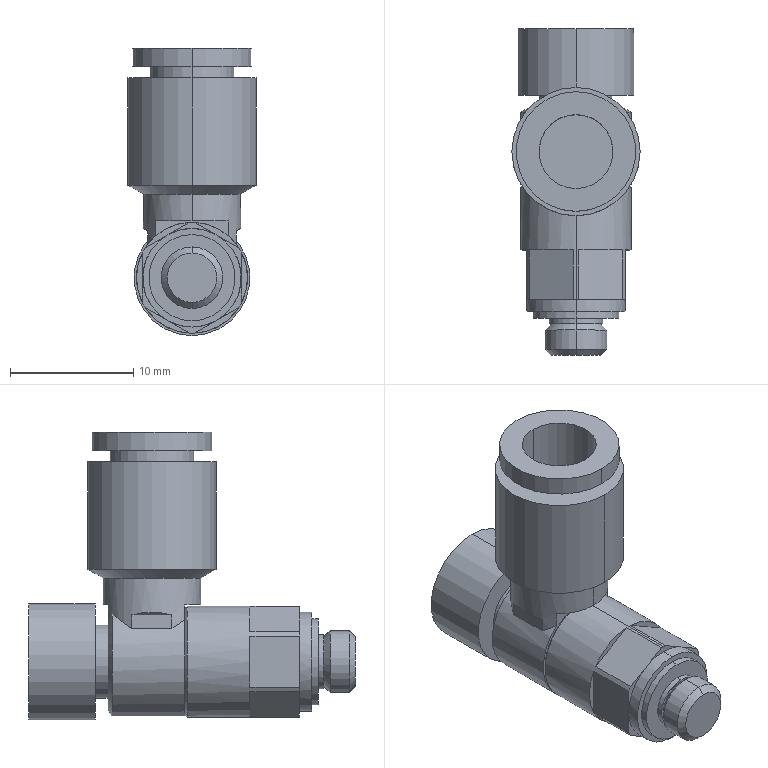Part | STEP file | speed control fitting AS1201FM-M5E-06A | 1 solid | 73 faces | box 10.4 x 26.5 x 23.3 mm | volume 2163 mm3 | plane 37 | cylinder 26 | cone 10 | commonest cylinder face diameters 9 x4 4.4 x2 5 x2 5.9 x2 6 x2 6.79 x2